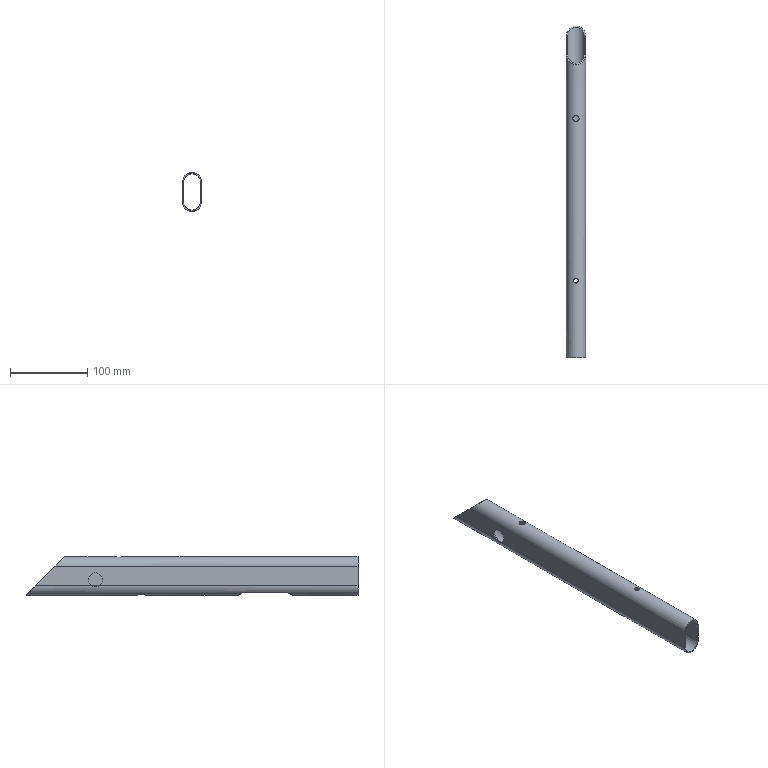Part | STEP file | 5091201L | 1 solid | 18 faces | box 25 x 430 x 50 mm | volume 72526 mm3 | cylinder 10 | plane 8 | commonest cylinder face diameters 18 x3 22 x2 25 x2 6 x1 8 x1 12 x1